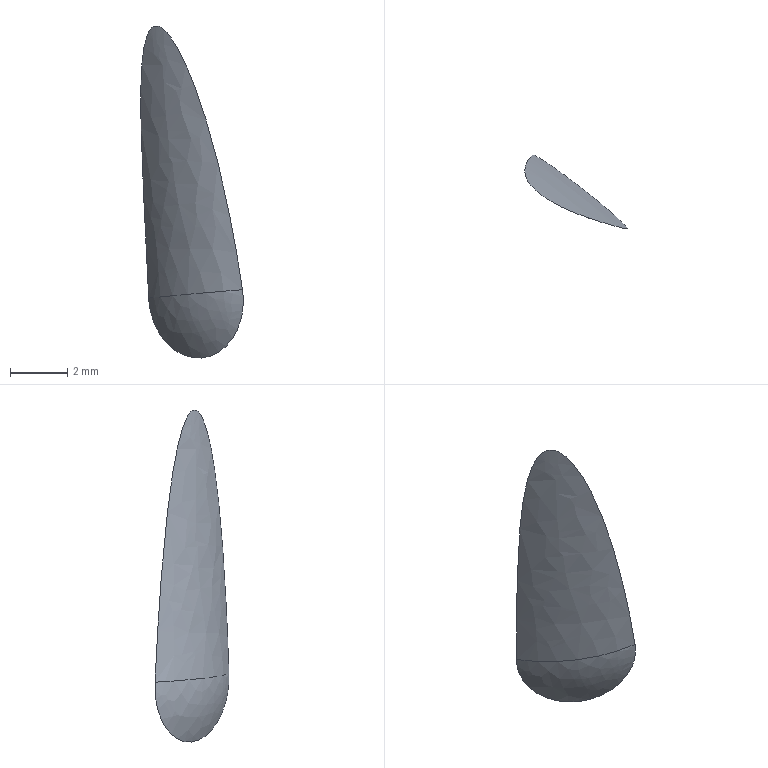Part | SolidWorks | features BaseBody 1 | 1 solid | 3 faces | box 3.595 x 2.597 x 11.642 mm | volume 8.157 mm3 | spline 3
STEP:
#1=CARTESIAN_POINT('',(82.211,90.498,-327.305));
#2=VERTEX_POINT('',#1);
#3=CARTESIAN_POINT('',(85.499,87.907,-327.008));
#4=VERTEX_POINT('',#3);
#5=CARTESIAN_POINT('',(82.211,90.498,-327.305));
#6=CARTESIAN_POINT('',(82.172,90.461,-326.471));
#7=CARTESIAN_POINT('',(82.131,90.417,-325.638));
#8=CARTESIAN_POINT('',(82.048,90.309,-323.973));
#9=CARTESIAN_POINT('',(82.007,90.246,-323.141));
#10=CARTESIAN_POINT('',(81.96,90.126,-321.894));
#11=CARTESIAN_POINT('',(81.947,90.081,-321.479));
#12=CARTESIAN_POINT('',(81.932,89.98,-320.651));
#13=CARTESIAN_POINT('',(81.929,89.922,-320.236));
#14=CARTESIAN_POINT('',(81.945,89.819,-319.619));
#15=CARTESIAN_POINT('',(81.953,89.782,-319.413));
#16=CARTESIAN_POINT('',(81.981,89.697,-319.005));
#17=CARTESIAN_POINT('',(82.001,89.651,-318.802));
#18=CARTESIAN_POINT('',(82.048,89.567,-318.504));
#19=CARTESIAN_POINT('',(82.066,89.537,-318.406));
#20=CARTESIAN_POINT('',(82.114,89.469,-318.213));
#21=CARTESIAN_POINT('',(82.143,89.432,-318.119));
#22=CARTESIAN_POINT('',(82.201,89.366,-317.989));
#23=CARTESIAN_POINT('',(82.223,89.342,-317.948));
#24=CARTESIAN_POINT('',(82.274,89.291,-317.873));
#25=CARTESIAN_POINT('',(82.304,89.262,-317.839));
#26=CARTESIAN_POINT('',(82.372,89.201,-317.787));
#27=CARTESIAN_POINT('',(82.411,89.169,-317.77));
#28=CARTESIAN_POINT('',(82.493,89.104,-317.76));
#29=CARTESIAN_POINT('',(82.536,89.072,-317.767));
#30=CARTESIAN_POINT('',(82.66,88.984,-317.813));
#31=CARTESIAN_POINT('',(82.734,88.937,-317.873));
#32=CARTESIAN_POINT('',(82.87,88.855,-318.009));
#33=CARTESIAN_POINT('',(82.931,88.82,-318.086));
#34=CARTESIAN_POINT('',(83.106,88.724,-318.328));
#35=CARTESIAN_POINT('',(83.206,88.675,-318.502));
#36=CARTESIAN_POINT('',(83.486,88.542,-319.038));
#37=CARTESIAN_POINT('',(83.646,88.476,-319.417));
#38=CARTESIAN_POINT('',(84.084,88.304,-320.565));
#39=CARTESIAN_POINT('',(84.322,88.226,-321.353));
#40=CARTESIAN_POINT('',(84.744,88.097,-322.949));
#41=CARTESIAN_POINT('',(84.925,88.048,-323.755));
#42=CARTESIAN_POINT('',(85.243,87.966,-325.374));
#43=CARTESIAN_POINT('',(85.38,87.933,-326.189));
#44=CARTESIAN_POINT('',(85.499,87.907,-327.008));
#45=B_SPLINE_CURVE_WITH_KNOTS('',3,(#5,#6,#7,#8,#9,#10,#11,#12,#13,#14,#15,#16,#17,#18,#19,#20,#21,#22,#23,#24,#25,#26,#27,#28,#29,#30,#31,#32,#33,#34,#35,#36,#37,#38,#39,#40,#41,#42,#43,#44),.UNSPECIFIED.,.F.,.F.,(4,2,2,2,2,2,2,2,2,2,2,2,2,2,2,2,2,2,2,4),(0.,0.002506,0.005012,0.006264,0.007517,0.008144,0.00877,0.009083,0.009397,0.009553,0.00971,0.009866,0.01002,0.01034,0.01065,0.01128,0.01253,0.01503,0.01754,0.02005),.UNSPECIFIED.);
#46=EDGE_CURVE('',#2,#4,#45,.T.);
#47=ORIENTED_EDGE('',*,*,#46,.T.);
#48=CARTESIAN_POINT('',(85.499,87.907,-327.008));
#49=CARTESIAN_POINT('',(85.52,87.902,-327.151));
#50=CARTESIAN_POINT('',(85.529,87.906,-327.294));
#51=CARTESIAN_POINT('',(85.525,87.933,-327.579));
#52=CARTESIAN_POINT('',(85.512,87.955,-327.723));
#53=CARTESIAN_POINT('',(85.463,88.017,-327.999));
#54=CARTESIAN_POINT('',(85.427,88.056,-328.132));
#55=CARTESIAN_POINT('',(85.335,88.15,-328.388));
#56=CARTESIAN_POINT('',(85.278,88.206,-328.51));
#57=CARTESIAN_POINT('',(85.08,88.389,-328.845));
#58=CARTESIAN_POINT('',(84.909,88.54,-329.032));
#59=CARTESIAN_POINT('',(84.618,88.784,-329.232));
#60=CARTESIAN_POINT('',(84.514,88.871,-329.286));
#61=CARTESIAN_POINT('',(84.299,89.045,-329.365));
#62=CARTESIAN_POINT('',(84.189,89.133,-329.39));
#63=CARTESIAN_POINT('',(83.964,89.311,-329.411));
#64=CARTESIAN_POINT('',(83.848,89.401,-329.406));
#65=CARTESIAN_POINT('',(83.623,89.573,-329.368));
#66=CARTESIAN_POINT('',(83.511,89.657,-329.334));
#67=CARTESIAN_POINT('',(83.291,89.819,-329.237));
#68=CARTESIAN_POINT('',(83.187,89.896,-329.175));
#69=CARTESIAN_POINT('',(82.987,90.038,-329.027));
#70=CARTESIAN_POINT('',(82.892,90.105,-328.938));
#71=CARTESIAN_POINT('',(82.718,90.223,-328.743));
#72=CARTESIAN_POINT('',(82.639,90.275,-328.635));
#73=CARTESIAN_POINT('',(82.498,90.365,-328.4));
#74=CARTESIAN_POINT('',(82.436,90.402,-328.274));
#75=CARTESIAN_POINT('',(82.284,90.487,-327.881));
#76=CARTESIAN_POINT('',(82.224,90.511,-327.594));
#77=CARTESIAN_POINT('',(82.211,90.498,-327.305));
#78=B_SPLINE_CURVE_WITH_KNOTS('',3,(#48,#49,#50,#51,#52,#53,#54,#55,#56,#57,#58,#59,#60,#61,#62,#63,#64,#65,#66,#67,#68,#69,#70,#71,#72,#73,#74,#75,#76,#77),.UNSPECIFIED.,.F.,.F.,(4,2,2,2,2,2,2,2,2,2,2,2,2,2,4),(0.,0.0004292,0.0008584,0.001288,0.001717,0.002575,0.003005,0.003434,0.003863,0.004292,0.004721,0.005151,0.00558,0.006009,0.006867),.UNSPECIFIED.);
#79=EDGE_CURVE('',#4,#2,#78,.T.);
#80=ORIENTED_EDGE('',*,*,#79,.T.);
#81=EDGE_LOOP('',(#47,#80));
#82=FACE_OUTER_BOUND('',#81,.T.);
#83=CARTESIAN_POINT('',(82.361,90.552,-329.766));
#84=CARTESIAN_POINT('',(83.527,89.68,-329.678));
#85=CARTESIAN_POINT('',(84.671,88.78,-329.591));
#86=CARTESIAN_POINT('',(85.793,87.851,-329.506));
#87=CARTESIAN_POINT('',(82.06,90.552,-325.784));
#88=CARTESIAN_POINT('',(83.222,89.68,-325.64));
#89=CARTESIAN_POINT('',(84.362,88.78,-325.498));
#90=CARTESIAN_POINT('',(85.479,87.851,-325.359));
#91=CARTESIAN_POINT('',(81.471,90.552,-321.835));
#92=CARTESIAN_POINT('',(82.624,89.68,-321.635));
#93=CARTESIAN_POINT('',(83.756,88.78,-321.438));
#94=CARTESIAN_POINT('',(84.866,87.851,-321.245));
#95=CARTESIAN_POINT('',(80.598,90.552,-317.939));
#96=CARTESIAN_POINT('',(81.739,89.68,-317.683));
#97=CARTESIAN_POINT('',(82.859,88.78,-317.432));
#98=CARTESIAN_POINT('',(83.956,87.851,-317.186));
#99=(BOUNDED_SURFACE()B_SPLINE_SURFACE(3,3,((#83,#84,#85,#86),(#87,#88,#89,#90),(#91,#92,#93,#94),(#95,#96,#97,#98)),.UNSPECIFIED.,.F.,.F.,.F.)B_SPLINE_SURFACE_WITH_KNOTS((4,4),(4,4),(0.,1.),(0.,1.),.UNSPECIFIED.)GEOMETRIC_REPRESENTATION_ITEM()RATIONAL_B_SPLINE_SURFACE(((1.001,1.001,1.001,1.001),(0.9997,0.9995,0.9995,0.9997),(0.9997,0.9995,0.9995,0.9997),(1.001,1.001,1.001,1.001)))REPRESENTATION_ITEM('')SURFACE());
#100=ADVANCED_FACE('',(#82),#99,.T.);
#101=ORIENTED_EDGE('',*,*,#79,.F.);
#102=CARTESIAN_POINT('',(85.499,87.907,-327.008));
#103=CARTESIAN_POINT('',(85.384,87.934,-327.017));
#104=CARTESIAN_POINT('',(85.243,87.971,-327.028));
#105=CARTESIAN_POINT('',(85.,88.052,-327.048));
#106=CARTESIAN_POINT('',(84.913,88.083,-327.056));
#107=CARTESIAN_POINT('',(84.776,88.138,-327.067));
#108=CARTESIAN_POINT('',(84.705,88.167,-327.073));
#109=CARTESIAN_POINT('',(84.619,88.204,-327.08));
#110=CARTESIAN_POINT('',(84.576,88.224,-327.084));
#111=CARTESIAN_POINT('',(84.554,88.234,-327.086));
#112=CARTESIAN_POINT('',(84.544,88.239,-327.087));
#113=CARTESIAN_POINT('',(84.538,88.242,-327.087));
#114=CARTESIAN_POINT('',(84.534,88.244,-327.088));
#115=CARTESIAN_POINT('',(84.401,88.306,-327.099));
#116=CARTESIAN_POINT('',(84.257,88.381,-327.111));
#117=CARTESIAN_POINT('',(84.026,88.518,-327.131));
#118=CARTESIAN_POINT('',(83.946,88.569,-327.138));
#119=CARTESIAN_POINT('',(83.823,88.652,-327.149));
#120=CARTESIAN_POINT('',(83.761,88.695,-327.155));
#121=CARTESIAN_POINT('',(83.688,88.749,-327.161));
#122=CARTESIAN_POINT('',(83.651,88.777,-327.165));
#123=CARTESIAN_POINT('',(83.632,88.791,-327.166));
#124=CARTESIAN_POINT('',(83.624,88.797,-327.167));
#125=CARTESIAN_POINT('',(83.619,88.801,-327.168));
#126=CARTESIAN_POINT('',(83.615,88.804,-327.168));
#127=CARTESIAN_POINT('',(83.4,88.97,-327.187));
#128=CARTESIAN_POINT('',(83.159,89.182,-327.209));
#129=CARTESIAN_POINT('',(82.671,89.736,-327.256));
#130=CARTESIAN_POINT('',(82.423,90.079,-327.281));
#131=CARTESIAN_POINT('',(82.211,90.498,-327.305));
#132=B_SPLINE_CURVE_WITH_KNOTS('',3,(#102,#103,#104,#105,#106,#107,#108,#109,#110,#111,#112,#113,#114,#115,#116,#117,#118,#119,#120,#121,#122,#123,#124,#125,#126,#127,#128,#129,#130,#131),.UNSPECIFIED.,.F.,.F.,(4,2,2,1,1,1,1,2,2,2,2,1,1,1,1,2,2,2,4),(0.,0.125,0.1875,0.2188,0.2344,0.2422,0.2461,0.248,0.25,0.375,0.4375,0.4688,0.4844,0.4922,0.4961,0.498,0.5,0.75,1.),.UNSPECIFIED.);
#133=EDGE_CURVE('',#4,#2,#132,.T.);
#134=ORIENTED_EDGE('',*,*,#133,.T.);
#135=EDGE_LOOP('',(#101,#134));
#136=FACE_OUTER_BOUND('',#135,.T.);
#137=CARTESIAN_POINT('',(85.555,87.894,-327.001));
#138=CARTESIAN_POINT('',(85.559,87.893,-327.325));
#139=CARTESIAN_POINT('',(85.696,87.892,-327.618));
#140=CARTESIAN_POINT('',(85.943,87.892,-327.827));
#141=CARTESIAN_POINT('',(84.068,88.228,-327.018));
#142=CARTESIAN_POINT('',(84.077,88.227,-327.78));
#143=CARTESIAN_POINT('',(84.401,88.225,-328.47));
#144=CARTESIAN_POINT('',(84.982,88.224,-328.962));
#145=CARTESIAN_POINT('',(82.868,89.167,-327.034));
#146=CARTESIAN_POINT('',(82.88,89.165,-328.15));
#147=CARTESIAN_POINT('',(83.355,89.162,-329.16));
#148=CARTESIAN_POINT('',(84.206,89.161,-329.881));
#149=CARTESIAN_POINT('',(82.184,90.53,-327.044));
#150=CARTESIAN_POINT('',(82.199,90.527,-328.362));
#151=CARTESIAN_POINT('',(82.759,90.524,-329.554));
#152=CARTESIAN_POINT('',(83.765,90.522,-330.405));
#153=(BOUNDED_SURFACE()B_SPLINE_SURFACE(3,3,((#137,#138,#139,#140),(#141,#142,#143,#144),(#145,#146,#147,#148),(#149,#150,#151,#152)),.UNSPECIFIED.,.F.,.F.,.T.)B_SPLINE_SURFACE_WITH_KNOTS((4,4),(4,4),(0.,1.),(0.,1.),.UNSPECIFIED.)GEOMETRIC_REPRESENTATION_ITEM()RATIONAL_B_SPLINE_SURFACE(((1.,0.9397,0.9397,1.),(0.9359,0.8795,0.8795,0.9359),(0.9359,0.8795,0.8795,0.9359),(1.,0.9397,0.9397,1.)))REPRESENTATION_ITEM('')SURFACE());
#154=ADVANCED_FACE('',(#136),#153,.T.);
#155=ORIENTED_EDGE('',*,*,#46,.F.);
#156=ORIENTED_EDGE('',*,*,#133,.F.);
#157=EDGE_LOOP('',(#155,#156));
#158=FACE_OUTER_BOUND('',#157,.T.);
#159=CARTESIAN_POINT('',(83.96,88.321,-317.384));
#160=CARTESIAN_POINT('',(82.653,88.747,-317.616));
#161=CARTESIAN_POINT('',(81.601,89.671,-317.833));
#162=CARTESIAN_POINT('',(81.014,90.974,-317.994));
#163=CARTESIAN_POINT('',(84.674,88.094,-320.593));
#164=CARTESIAN_POINT('',(83.304,88.481,-320.807));
#165=CARTESIAN_POINT('',(82.183,89.406,-320.996));
#166=CARTESIAN_POINT('',(81.549,90.748,-321.122));
#167=CARTESIAN_POINT('',(85.206,87.97,-323.832));
#168=CARTESIAN_POINT('',(83.785,88.324,-323.999));
#169=CARTESIAN_POINT('',(82.611,89.247,-324.149));
#170=CARTESIAN_POINT('',(81.943,90.617,-324.249));
#171=CARTESIAN_POINT('',(85.551,87.895,-327.1));
#172=CARTESIAN_POINT('',(84.097,88.226,-327.216));
#173=CARTESIAN_POINT('',(82.888,89.147,-327.324));
#174=CARTESIAN_POINT('',(82.199,90.534,-327.4));
#175=(BOUNDED_SURFACE()B_SPLINE_SURFACE(3,3,((#159,#160,#161,#162),(#163,#164,#165,#166),(#167,#168,#169,#170),(#171,#172,#173,#174)),.UNSPECIFIED.,.F.,.F.,.F.)B_SPLINE_SURFACE_WITH_KNOTS((4,4),(4,4),(-0.003716,1.01),(-0.004112,1.003),.UNSPECIFIED.)GEOMETRIC_REPRESENTATION_ITEM()RATIONAL_B_SPLINE_SURFACE(((0.9968,0.9144,0.8861,0.9117),(0.9966,0.9092,0.8792,0.9064),(0.9964,0.9052,0.8738,0.9022),(0.9963,0.9026,0.8703,0.8995)))REPRESENTATION_ITEM('')SURFACE());
#176=ADVANCED_FACE('',(#158),#175,.F.);
#177=CLOSED_SHELL('',(#100,#154,#176));
#178=MANIFOLD_SOLID_BREP('',#177);
#179=CARTESIAN_POINT('',(0.,0.,0.));
#180=DIRECTION('',(0.,0.,1.));
#181=DIRECTION('',(1.,0.,0.));
#182=AXIS2_PLACEMENT_3D('',#179,#180,#181);
#183=(LENGTH_UNIT()NAMED_UNIT(*)SI_UNIT(.MILLI.,.METRE.));
#184=UNCERTAINTY_MEASURE_WITH_UNIT(LENGTH_MEASURE(0.00001),#183,'','');
#185=(NAMED_UNIT(*)PLANE_ANGLE_UNIT()SI_UNIT($,.RADIAN.));
#186=(NAMED_UNIT(*)SI_UNIT($,.STERADIAN.)SOLID_ANGLE_UNIT());
#187=(GEOMETRIC_REPRESENTATION_CONTEXT(3)GLOBAL_UNCERTAINTY_ASSIGNED_CONTEXT((#184))GLOBAL_UNIT_ASSIGNED_CONTEXT((#183,#185,#186))REPRESENTATION_CONTEXT('',''));
#188=ADVANCED_BREP_SHAPE_REPRESENTATION('',(#178,#182),#187);